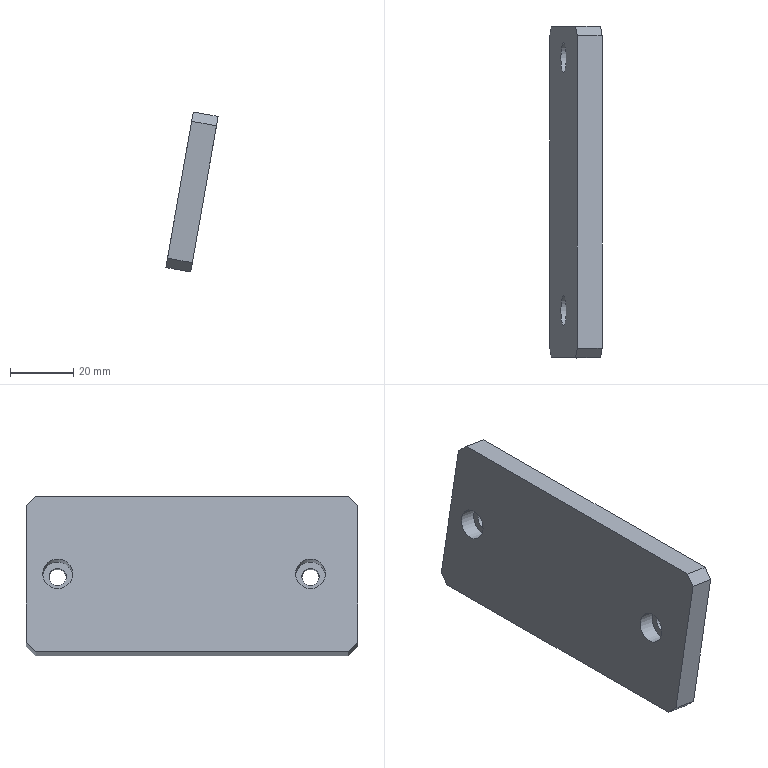Part | STEP file | P011002S003-006 | 1 solid | 16 faces | box 16.561 x 105 x 50.63 mm | volume 40958 mm3 | plane 12 | cylinder 4 | commonest cylinder face diameters 5.5 x2 9.5 x2
STEP:
#1=CARTESIAN_POINT('',(0.,0.,0.));
#2=DIRECTION('',(0.,0.,1.));
#3=DIRECTION('',(1.,0.,0.));
#4=AXIS2_PLACEMENT_3D('',#1,#2,#3);
#5=CARTESIAN_POINT('',(-223.214,6.,16.938));
#6=VERTEX_POINT('',#5);
#7=CARTESIAN_POINT('',(-223.692,6.,14.229));
#8=DIRECTION('',(0.9848,0.,-0.1736));
#9=DIRECTION('',(0.1736,0.,0.9848));
#10=AXIS2_PLACEMENT_3D('',#7,#8,#9);
#11=CIRCLE('',#10,2.75);
#12=CARTESIAN_POINT('',(-220.219,-62.,33.926));
#13=DIRECTION('',(0.9848,0.,-0.1736));
#14=DIRECTION('',(0.,1.,0.));
#15=AXIS2_PLACEMENT_3D('',#12,#13,#14);
#16=PLANE('',#15);
#17=CARTESIAN_POINT('',(68.,-20.));
#18=DIRECTION('',(0.,1.));
#19=AXIS2_PLACEMENT_2D('',#17,#18);
#20=CIRCLE('',#19,2.75);
#21=(GEOMETRIC_REPRESENTATION_CONTEXT(2)PARAMETRIC_REPRESENTATION_CONTEXT()REPRESENTATION_CONTEXT('',''));
#22=DEFINITIONAL_REPRESENTATION('',(#20),#21);
#23=PCURVE('',#16,#22);
#24=CARTESIAN_POINT('',(-231.57,6.,15.619));
#25=DIRECTION('',(0.9848,0.,-0.1736));
#26=DIRECTION('',(0.1736,0.,0.9848));
#27=AXIS2_PLACEMENT_3D('',#24,#25,#26);
#28=CYLINDRICAL_SURFACE('',#27,2.75);
#29=CARTESIAN_POINT('',(0.,8.));
#30=DIRECTION('',(1.,0.));
#31=VECTOR('',#30,1.);
#32=LINE('',#29,#31);
#33=(GEOMETRIC_REPRESENTATION_CONTEXT(2)PARAMETRIC_REPRESENTATION_CONTEXT()REPRESENTATION_CONTEXT('',''));
#34=DEFINITIONAL_REPRESENTATION('',(#32),#33);
#35=PCURVE('',#28,#34);
#36=SURFACE_CURVE('',#11,(#23,#35),.PCURVE_S1.);
#37=EDGE_CURVE('',#6,#6,#36,.T.);
#38=ORIENTED_EDGE('',*,*,#37,.F.);
#39=EDGE_LOOP('',(#38));
#40=FACE_BOUND('',#39,.T.);
#41=CARTESIAN_POINT('',(-219.35,93.,38.85));
#42=VERTEX_POINT('',#41);
#43=CARTESIAN_POINT('',(-219.35,-6.,38.85));
#44=VERTEX_POINT('',#43);
#45=CARTESIAN_POINT('',(-219.35,-62.,38.85));
#46=DIRECTION('',(0.,-1.,0.));
#47=VECTOR('',#46,1.);
#48=LINE('',#45,#47);
#49=CARTESIAN_POINT('',(0.,5.));
#50=DIRECTION('',(-1.,0.));
#51=VECTOR('',#50,1.);
#52=LINE('',#49,#51);
#53=(GEOMETRIC_REPRESENTATION_CONTEXT(2)PARAMETRIC_REPRESENTATION_CONTEXT()REPRESENTATION_CONTEXT('',''));
#54=DEFINITIONAL_REPRESENTATION('',(#52),#53);
#55=PCURVE('',#16,#54);
#56=CARTESIAN_POINT('',(-226.736,-62.,40.152));
#57=DIRECTION('',(0.1736,0.,0.9848));
#58=DIRECTION('',(0.9848,0.,-0.1736));
#59=AXIS2_PLACEMENT_3D('',#56,#57,#58);
#60=PLANE('',#59);
#61=CARTESIAN_POINT('',(7.5,0.));
#62=DIRECTION('',(0.,-1.));
#63=VECTOR('',#62,1.);
#64=LINE('',#61,#63);
#65=(GEOMETRIC_REPRESENTATION_CONTEXT(2)PARAMETRIC_REPRESENTATION_CONTEXT()REPRESENTATION_CONTEXT('',''));
#66=DEFINITIONAL_REPRESENTATION('',(#64),#65);
#67=PCURVE('',#60,#66);
#68=SURFACE_CURVE('',#48,(#55,#67),.PCURVE_S1.);
#69=EDGE_CURVE('',#42,#44,#68,.T.);
#70=ORIENTED_EDGE('',*,*,#69,.T.);
#71=CARTESIAN_POINT('',(-219.871,-9.,35.895));
#72=VERTEX_POINT('',#71);
#73=CARTESIAN_POINT('',(-224.647,-36.5,8.813));
#74=DIRECTION('',(0.1228,0.7071,0.6964));
#75=VECTOR('',#74,1.);
#76=LINE('',#73,#75);
#77=CARTESIAN_POINT('',(25.5,-25.5));
#78=DIRECTION('',(0.7071,0.7071));
#79=VECTOR('',#78,1.);
#80=LINE('',#77,#79);
#81=(GEOMETRIC_REPRESENTATION_CONTEXT(2)PARAMETRIC_REPRESENTATION_CONTEXT()REPRESENTATION_CONTEXT('',''));
#82=DEFINITIONAL_REPRESENTATION('',(#80),#81);
#83=PCURVE('',#16,#82);
#84=CARTESIAN_POINT('',(-200.102,-9.,32.409));
#85=DIRECTION('',(0.1228,-0.7071,0.6964));
#86=DIRECTION('',(0.,-0.7017,-0.7125));
#87=AXIS2_PLACEMENT_3D('',#84,#85,#86);
#88=PLANE('',#87);
#89=CARTESIAN_POINT('',(36.108,-24.732));
#90=DIRECTION('',(-0.9923,0.1237));
#91=VECTOR('',#90,1.);
#92=LINE('',#89,#91);
#93=(GEOMETRIC_REPRESENTATION_CONTEXT(2)PARAMETRIC_REPRESENTATION_CONTEXT()REPRESENTATION_CONTEXT('',''));
#94=DEFINITIONAL_REPRESENTATION('',(#92),#93);
#95=PCURVE('',#88,#94);
#96=SURFACE_CURVE('',#76,(#83,#95),.PCURVE_S1.);
#97=EDGE_CURVE('',#72,#44,#96,.T.);
#98=ORIENTED_EDGE('',*,*,#97,.F.);
#99=CARTESIAN_POINT('',(-227.512,-9.,-7.436));
#100=VERTEX_POINT('',#99);
#101=CARTESIAN_POINT('',(-220.219,-9.,33.926));
#102=DIRECTION('',(-0.1736,0.,-0.9848));
#103=VECTOR('',#102,1.);
#104=LINE('',#101,#103);
#105=CARTESIAN_POINT('',(53.,0.));
#106=DIRECTION('',(0.,-1.));
#107=VECTOR('',#106,1.);
#108=LINE('',#105,#107);
#109=(GEOMETRIC_REPRESENTATION_CONTEXT(2)PARAMETRIC_REPRESENTATION_CONTEXT()REPRESENTATION_CONTEXT('',''));
#110=DEFINITIONAL_REPRESENTATION('',(#108),#109);
#111=PCURVE('',#16,#110);
#112=CARTESIAN_POINT('',(-197.,-9.,50.));
#113=DIRECTION('',(0.,1.,0.));
#114=DIRECTION('',(0.,0.,1.));
#115=AXIS2_PLACEMENT_3D('',#112,#113,#114);
#116=PLANE('',#115);
#117=CARTESIAN_POINT('',(-16.074,-23.219));
#118=DIRECTION('',(-0.9848,-0.1736));
#119=VECTOR('',#118,1.);
#120=LINE('',#117,#119);
#121=(GEOMETRIC_REPRESENTATION_CONTEXT(2)PARAMETRIC_REPRESENTATION_CONTEXT()REPRESENTATION_CONTEXT('',''));
#122=DEFINITIONAL_REPRESENTATION('',(#120),#121);
#123=PCURVE('',#116,#122);
#124=SURFACE_CURVE('',#104,(#111,#123),.PCURVE_S1.);
#125=EDGE_CURVE('',#72,#100,#124,.T.);
#126=ORIENTED_EDGE('',*,*,#125,.T.);
#127=CARTESIAN_POINT('',(-228.033,-6.,-10.391));
#128=VERTEX_POINT('',#127);
#129=CARTESIAN_POINT('',(-219.264,-56.5,39.342));
#130=DIRECTION('',(0.1228,-0.7071,0.6964));
#131=VECTOR('',#130,1.);
#132=LINE('',#129,#131);
#133=CARTESIAN_POINT('',(5.5,5.5));
#134=DIRECTION('',(-0.7071,0.7071));
#135=VECTOR('',#134,1.);
#136=LINE('',#133,#135);
#137=(GEOMETRIC_REPRESENTATION_CONTEXT(2)PARAMETRIC_REPRESENTATION_CONTEXT()REPRESENTATION_CONTEXT('',''));
#138=DEFINITIONAL_REPRESENTATION('',(#136),#137);
#139=PCURVE('',#16,#138);
#140=CARTESIAN_POINT('',(-207.742,-9.,-10.922));
#141=DIRECTION('',(-0.1228,-0.7071,-0.6964));
#142=DIRECTION('',(0.,0.7017,-0.7125));
#143=AXIS2_PLACEMENT_3D('',#140,#141,#142);
#144=PLANE('',#143);
#145=CARTESIAN_POINT('',(-69.143,-11.609));
#146=DIRECTION('',(-0.9923,0.1237));
#147=VECTOR('',#146,1.);
#148=LINE('',#145,#147);
#149=(GEOMETRIC_REPRESENTATION_CONTEXT(2)PARAMETRIC_REPRESENTATION_CONTEXT()REPRESENTATION_CONTEXT('',''));
#150=DEFINITIONAL_REPRESENTATION('',(#148),#149);
#151=PCURVE('',#144,#150);
#152=SURFACE_CURVE('',#132,(#139,#151),.PCURVE_S1.);
#153=EDGE_CURVE('',#128,#100,#152,.T.);
#154=ORIENTED_EDGE('',*,*,#153,.F.);
#155=CARTESIAN_POINT('',(-228.033,93.,-10.391));
#156=VERTEX_POINT('',#155);
#157=CARTESIAN_POINT('',(-228.033,-62.,-10.391));
#158=DIRECTION('',(0.,1.,0.));
#159=VECTOR('',#158,1.);
#160=LINE('',#157,#159);
#161=CARTESIAN_POINT('',(0.,-45.));
#162=DIRECTION('',(1.,0.));
#163=VECTOR('',#162,1.);
#164=LINE('',#161,#163);
#165=(GEOMETRIC_REPRESENTATION_CONTEXT(2)PARAMETRIC_REPRESENTATION_CONTEXT()REPRESENTATION_CONTEXT('',''));
#166=DEFINITIONAL_REPRESENTATION('',(#164),#165);
#167=PCURVE('',#16,#166);
#168=CARTESIAN_POINT('',(-235.419,-62.,-9.088));
#169=DIRECTION('',(-0.1736,0.,-0.9848));
#170=DIRECTION('',(-0.9848,0.,0.1736));
#171=AXIS2_PLACEMENT_3D('',#168,#169,#170);
#172=PLANE('',#171);
#173=CARTESIAN_POINT('',(-7.5,0.));
#174=DIRECTION('',(0.,1.));
#175=VECTOR('',#174,1.);
#176=LINE('',#173,#175);
#177=(GEOMETRIC_REPRESENTATION_CONTEXT(2)PARAMETRIC_REPRESENTATION_CONTEXT()REPRESENTATION_CONTEXT('',''));
#178=DEFINITIONAL_REPRESENTATION('',(#176),#177);
#179=PCURVE('',#172,#178);
#180=SURFACE_CURVE('',#160,(#167,#179),.PCURVE_S1.);
#181=EDGE_CURVE('',#128,#156,#180,.T.);
#182=ORIENTED_EDGE('',*,*,#181,.T.);
#183=CARTESIAN_POINT('',(-227.512,96.,-7.436));
#184=VERTEX_POINT('',#183);
#185=CARTESIAN_POINT('',(-237.583,38.,-64.555));
#186=DIRECTION('',(-0.1228,-0.7071,-0.6964));
#187=VECTOR('',#186,1.);
#188=LINE('',#185,#187);
#189=CARTESIAN_POINT('',(100.,-100.));
#190=DIRECTION('',(-0.7071,-0.7071));
#191=VECTOR('',#190,1.);
#192=LINE('',#189,#191);
#193=(GEOMETRIC_REPRESENTATION_CONTEXT(2)PARAMETRIC_REPRESENTATION_CONTEXT()REPRESENTATION_CONTEXT('',''));
#194=DEFINITIONAL_REPRESENTATION('',(#192),#193);
#195=PCURVE('',#16,#194);
#196=CARTESIAN_POINT('',(-231.451,96.,-6.742));
#197=DIRECTION('',(-0.1228,0.7071,-0.6964));
#198=DIRECTION('',(0.,0.7017,0.7125));
#199=AXIS2_PLACEMENT_3D('',#196,#197,#198);
#200=PLANE('',#199);
#201=CARTESIAN_POINT('',(-81.889,-6.179));
#202=DIRECTION('',(-0.9923,-0.1237));
#203=VECTOR('',#202,1.);
#204=LINE('',#201,#203);
#205=(GEOMETRIC_REPRESENTATION_CONTEXT(2)PARAMETRIC_REPRESENTATION_CONTEXT()REPRESENTATION_CONTEXT('',''));
#206=DEFINITIONAL_REPRESENTATION('',(#204),#205);
#207=PCURVE('',#200,#206);
#208=SURFACE_CURVE('',#188,(#195,#207),.PCURVE_S1.);
#209=EDGE_CURVE('',#184,#156,#208,.T.);
#210=ORIENTED_EDGE('',*,*,#209,.F.);
#211=CARTESIAN_POINT('',(-219.871,96.,35.895));
#212=VERTEX_POINT('',#211);
#213=CARTESIAN_POINT('',(-220.219,96.,33.926));
#214=DIRECTION('',(0.1736,0.,0.9848));
#215=VECTOR('',#214,1.);
#216=LINE('',#213,#215);
#217=CARTESIAN_POINT('',(158.,0.));
#218=DIRECTION('',(0.,1.));
#219=VECTOR('',#218,1.);
#220=LINE('',#217,#219);
#221=(GEOMETRIC_REPRESENTATION_CONTEXT(2)PARAMETRIC_REPRESENTATION_CONTEXT()REPRESENTATION_CONTEXT('',''));
#222=DEFINITIONAL_REPRESENTATION('',(#220),#221);
#223=PCURVE('',#16,#222);
#224=CARTESIAN_POINT('',(-227.631,96.,14.924));
#225=DIRECTION('',(0.,-1.,0.));
#226=DIRECTION('',(0.,0.,-1.));
#227=AXIS2_PLACEMENT_3D('',#224,#225,#226);
#228=PLANE('',#227);
#229=CARTESIAN_POINT('',(-19.002,7.412));
#230=DIRECTION('',(-0.9848,0.1736));
#231=VECTOR('',#230,1.);
#232=LINE('',#229,#231);
#233=(GEOMETRIC_REPRESENTATION_CONTEXT(2)PARAMETRIC_REPRESENTATION_CONTEXT()REPRESENTATION_CONTEXT('',''));
#234=DEFINITIONAL_REPRESENTATION('',(#232),#233);
#235=PCURVE('',#228,#234);
#236=SURFACE_CURVE('',#216,(#223,#235),.PCURVE_S1.);
#237=EDGE_CURVE('',#184,#212,#236,.T.);
#238=ORIENTED_EDGE('',*,*,#237,.T.);
#239=CARTESIAN_POINT('',(-206.327,18.,112.71));
#240=DIRECTION('',(-0.1228,0.7071,-0.6964));
#241=VECTOR('',#240,1.);
#242=LINE('',#239,#241);
#243=CARTESIAN_POINT('',(80.,80.));
#244=DIRECTION('',(0.7071,-0.7071));
#245=VECTOR('',#244,1.);
#246=LINE('',#243,#245);
#247=(GEOMETRIC_REPRESENTATION_CONTEXT(2)PARAMETRIC_REPRESENTATION_CONTEXT()REPRESENTATION_CONTEXT('',''));
#248=DEFINITIONAL_REPRESENTATION('',(#246),#247);
#249=PCURVE('',#16,#248);
#250=CARTESIAN_POINT('',(-223.811,96.,36.59));
#251=DIRECTION('',(0.1228,0.7071,0.6964));
#252=DIRECTION('',(0.,-0.7017,0.7125));
#253=AXIS2_PLACEMENT_3D('',#250,#251,#252);
#254=PLANE('',#253);
#255=CARTESIAN_POINT('',(108.966,17.617));
#256=DIRECTION('',(-0.9923,-0.1237));
#257=VECTOR('',#256,1.);
#258=LINE('',#255,#257);
#259=(GEOMETRIC_REPRESENTATION_CONTEXT(2)PARAMETRIC_REPRESENTATION_CONTEXT()REPRESENTATION_CONTEXT('',''));
#260=DEFINITIONAL_REPRESENTATION('',(#258),#259);
#261=PCURVE('',#254,#260);
#262=SURFACE_CURVE('',#242,(#249,#261),.PCURVE_S1.);
#263=EDGE_CURVE('',#42,#212,#262,.T.);
#264=ORIENTED_EDGE('',*,*,#263,.F.);
#265=EDGE_LOOP('',(#70,#98,#126,#154,#182,#210,#238,#264));
#266=FACE_BOUND('',#265,.T.);
#267=CARTESIAN_POINT('',(-223.214,86.,16.938));
#268=VERTEX_POINT('',#267);
#269=CARTESIAN_POINT('',(-223.692,86.,14.229));
#270=DIRECTION('',(0.9848,0.,-0.1736));
#271=DIRECTION('',(0.1736,0.,0.9848));
#272=AXIS2_PLACEMENT_3D('',#269,#270,#271);
#273=CIRCLE('',#272,2.75);
#274=CARTESIAN_POINT('',(148.,-20.));
#275=DIRECTION('',(0.,1.));
#276=AXIS2_PLACEMENT_2D('',#274,#275);
#277=CIRCLE('',#276,2.75);
#278=(GEOMETRIC_REPRESENTATION_CONTEXT(2)PARAMETRIC_REPRESENTATION_CONTEXT()REPRESENTATION_CONTEXT('',''));
#279=DEFINITIONAL_REPRESENTATION('',(#277),#278);
#280=PCURVE('',#16,#279);
#281=CARTESIAN_POINT('',(-231.57,86.,15.619));
#282=DIRECTION('',(0.9848,0.,-0.1736));
#283=DIRECTION('',(0.1736,0.,0.9848));
#284=AXIS2_PLACEMENT_3D('',#281,#282,#283);
#285=CYLINDRICAL_SURFACE('',#284,2.75);
#286=CARTESIAN_POINT('',(0.,8.));
#287=DIRECTION('',(1.,0.));
#288=VECTOR('',#287,1.);
#289=LINE('',#286,#288);
#290=(GEOMETRIC_REPRESENTATION_CONTEXT(2)PARAMETRIC_REPRESENTATION_CONTEXT()REPRESENTATION_CONTEXT('',''));
#291=DEFINITIONAL_REPRESENTATION('',(#289),#290);
#292=PCURVE('',#285,#291);
#293=SURFACE_CURVE('',#273,(#280,#292),.PCURVE_S1.);
#294=EDGE_CURVE('',#268,#268,#293,.T.);
#295=ORIENTED_EDGE('',*,*,#294,.F.);
#296=EDGE_LOOP('',(#295));
#297=FACE_BOUND('',#296,.T.);
#298=ADVANCED_FACE('',(#40,#266,#297),#16,.T.);
#299=CARTESIAN_POINT('',(-230.745,86.,20.296));
#300=VERTEX_POINT('',#299);
#301=CARTESIAN_POINT('',(-231.57,86.,15.619));
#302=DIRECTION('',(0.9848,0.,-0.1736));
#303=DIRECTION('',(0.1736,0.,0.9848));
#304=AXIS2_PLACEMENT_3D('',#301,#302,#303);
#305=CIRCLE('',#304,4.75);
#306=CARTESIAN_POINT('',(-228.097,-62.,35.315));
#307=DIRECTION('',(-0.9848,0.,0.1736));
#308=DIRECTION('',(0.,-1.,0.));
#309=AXIS2_PLACEMENT_3D('',#306,#307,#308);
#310=PLANE('',#309);
#311=CARTESIAN_POINT('',(-148.,-15.25));
#312=CARTESIAN_POINT('',(-139.773,-15.25));
#313=CARTESIAN_POINT('',(-143.886,-22.375));
#314=CARTESIAN_POINT('',(-148.,-29.5));
#315=CARTESIAN_POINT('',(-152.114,-22.375));
#316=CARTESIAN_POINT('',(-156.227,-15.25));
#317=CARTESIAN_POINT('',(-148.,-15.25));
#318=(BOUNDED_CURVE()B_SPLINE_CURVE(2,(#311,#312,#313,#314,#315,#316,#317),.UNSPECIFIED.,.T.,.F.)B_SPLINE_CURVE_WITH_KNOTS((1,2,2,2,2,1),(-2.094,0.,2.094,4.189,6.283,8.378),.UNSPECIFIED.)CURVE()GEOMETRIC_REPRESENTATION_ITEM()RATIONAL_B_SPLINE_CURVE((1.,0.5,1.,0.5,1.,0.5,1.))REPRESENTATION_ITEM(''));
#319=(GEOMETRIC_REPRESENTATION_CONTEXT(2)PARAMETRIC_REPRESENTATION_CONTEXT()REPRESENTATION_CONTEXT('',''));
#320=DEFINITIONAL_REPRESENTATION('',(#318),#319);
#321=PCURVE('',#310,#320);
#322=CARTESIAN_POINT('',(-231.57,86.,15.619));
#323=DIRECTION('',(0.9848,0.,-0.1736));
#324=DIRECTION('',(0.1736,0.,0.9848));
#325=AXIS2_PLACEMENT_3D('',#322,#323,#324);
#326=CYLINDRICAL_SURFACE('',#325,4.75);
#327=CARTESIAN_POINT('',(0.,0.));
#328=DIRECTION('',(1.,0.));
#329=VECTOR('',#328,1.);
#330=LINE('',#327,#329);
#331=(GEOMETRIC_REPRESENTATION_CONTEXT(2)PARAMETRIC_REPRESENTATION_CONTEXT()REPRESENTATION_CONTEXT('',''));
#332=DEFINITIONAL_REPRESENTATION('',(#330),#331);
#333=PCURVE('',#326,#332);
#334=SURFACE_CURVE('',#305,(#321,#333),.PCURVE_S1.);
#335=EDGE_CURVE('',#300,#300,#334,.T.);
#336=ORIENTED_EDGE('',*,*,#335,.T.);
#337=EDGE_LOOP('',(#336));
#338=FACE_BOUND('',#337,.T.);
#339=CARTESIAN_POINT('',(-230.745,6.,20.296));
#340=VERTEX_POINT('',#339);
#341=CARTESIAN_POINT('',(-231.57,6.,15.619));
#342=DIRECTION('',(0.9848,0.,-0.1736));
#343=DIRECTION('',(0.1736,0.,0.9848));
#344=AXIS2_PLACEMENT_3D('',#341,#342,#343);
#345=CIRCLE('',#344,4.75);
#346=CARTESIAN_POINT('',(-68.,-15.25));
#347=CARTESIAN_POINT('',(-59.773,-15.25));
#348=CARTESIAN_POINT('',(-63.886,-22.375));
#349=CARTESIAN_POINT('',(-68.,-29.5));
#350=CARTESIAN_POINT('',(-72.114,-22.375));
#351=CARTESIAN_POINT('',(-76.227,-15.25));
#352=CARTESIAN_POINT('',(-68.,-15.25));
#353=(BOUNDED_CURVE()B_SPLINE_CURVE(2,(#346,#347,#348,#349,#350,#351,#352),.UNSPECIFIED.,.T.,.F.)B_SPLINE_CURVE_WITH_KNOTS((1,2,2,2,2,1),(-2.094,0.,2.094,4.189,6.283,8.378),.UNSPECIFIED.)CURVE()GEOMETRIC_REPRESENTATION_ITEM()RATIONAL_B_SPLINE_CURVE((1.,0.5,1.,0.5,1.,0.5,1.))REPRESENTATION_ITEM(''));
#354=(GEOMETRIC_REPRESENTATION_CONTEXT(2)PARAMETRIC_REPRESENTATION_CONTEXT()REPRESENTATION_CONTEXT('',''));
#355=DEFINITIONAL_REPRESENTATION('',(#353),#354);
#356=PCURVE('',#310,#355);
#357=CARTESIAN_POINT('',(-231.57,6.,15.619));
#358=DIRECTION('',(0.9848,0.,-0.1736));
#359=DIRECTION('',(0.1736,0.,0.9848));
#360=AXIS2_PLACEMENT_3D('',#357,#358,#359);
#361=CYLINDRICAL_SURFACE('',#360,4.75);
#362=CARTESIAN_POINT('',(0.,0.));
#363=DIRECTION('',(1.,0.));
#364=VECTOR('',#363,1.);
#365=LINE('',#362,#364);
#366=(GEOMETRIC_REPRESENTATION_CONTEXT(2)PARAMETRIC_REPRESENTATION_CONTEXT()REPRESENTATION_CONTEXT('',''));
#367=DEFINITIONAL_REPRESENTATION('',(#365),#366);
#368=PCURVE('',#361,#367);
#369=SURFACE_CURVE('',#345,(#356,#368),.PCURVE_S1.);
#370=EDGE_CURVE('',#340,#340,#369,.T.);
#371=ORIENTED_EDGE('',*,*,#370,.T.);
#372=EDGE_LOOP('',(#371));
#373=FACE_BOUND('',#372,.T.);
#374=CARTESIAN_POINT('',(-227.75,96.,37.284));
#375=VERTEX_POINT('',#374);
#376=CARTESIAN_POINT('',(-235.39,96.,-6.047));
#377=VERTEX_POINT('',#376);
#378=CARTESIAN_POINT('',(-228.097,96.,35.315));
#379=DIRECTION('',(-0.1736,0.,-0.9848));
#380=VECTOR('',#379,1.);
#381=LINE('',#378,#380);
#382=CARTESIAN_POINT('',(-158.,0.));
#383=DIRECTION('',(0.,-1.));
#384=VECTOR('',#383,1.);
#385=LINE('',#382,#384);
#386=(GEOMETRIC_REPRESENTATION_CONTEXT(2)PARAMETRIC_REPRESENTATION_CONTEXT()REPRESENTATION_CONTEXT('',''));
#387=DEFINITIONAL_REPRESENTATION('',(#385),#386);
#388=PCURVE('',#310,#387);
#389=CARTESIAN_POINT('',(-20.391,-0.4663));
#390=DIRECTION('',(0.9848,-0.1736));
#391=VECTOR('',#390,1.);
#392=LINE('',#389,#391);
#393=(GEOMETRIC_REPRESENTATION_CONTEXT(2)PARAMETRIC_REPRESENTATION_CONTEXT()REPRESENTATION_CONTEXT('',''));
#394=DEFINITIONAL_REPRESENTATION('',(#392),#393);
#395=PCURVE('',#228,#394);
#396=SURFACE_CURVE('',#381,(#388,#395),.PCURVE_S1.);
#397=EDGE_CURVE('',#375,#377,#396,.T.);
#398=ORIENTED_EDGE('',*,*,#397,.T.);
#399=CARTESIAN_POINT('',(-235.911,93.,-9.002));
#400=VERTEX_POINT('',#399);
#401=CARTESIAN_POINT('',(-245.462,38.,-63.166));
#402=DIRECTION('',(0.1228,0.7071,0.6964));
#403=VECTOR('',#402,1.);
#404=LINE('',#401,#403);
#405=CARTESIAN_POINT('',(-100.,-100.));
#406=DIRECTION('',(-0.7071,0.7071));
#407=VECTOR('',#406,1.);
#408=LINE('',#405,#407);
#409=(GEOMETRIC_REPRESENTATION_CONTEXT(2)PARAMETRIC_REPRESENTATION_CONTEXT()REPRESENTATION_CONTEXT('',''));
#410=DEFINITIONAL_REPRESENTATION('',(#408),#409);
#411=PCURVE('',#310,#410);
#412=CARTESIAN_POINT('',(-80.899,-14.118));
#413=DIRECTION('',(0.9923,0.1237));
#414=VECTOR('',#413,1.);
#415=LINE('',#412,#414);
#416=(GEOMETRIC_REPRESENTATION_CONTEXT(2)PARAMETRIC_REPRESENTATION_CONTEXT()REPRESENTATION_CONTEXT('',''));
#417=DEFINITIONAL_REPRESENTATION('',(#415),#416);
#418=PCURVE('',#200,#417);
#419=SURFACE_CURVE('',#404,(#411,#418),.PCURVE_S1.);
#420=EDGE_CURVE('',#400,#377,#419,.T.);
#421=ORIENTED_EDGE('',*,*,#420,.F.);
#422=CARTESIAN_POINT('',(-235.911,-6.,-9.002));
#423=VERTEX_POINT('',#422);
#424=CARTESIAN_POINT('',(-235.911,-62.,-9.002));
#425=DIRECTION('',(0.,-1.,0.));
#426=VECTOR('',#425,1.);
#427=LINE('',#424,#426);
#428=CARTESIAN_POINT('',(0.,-45.));
#429=DIRECTION('',(1.,0.));
#430=VECTOR('',#429,1.);
#431=LINE('',#428,#430);
#432=(GEOMETRIC_REPRESENTATION_CONTEXT(2)PARAMETRIC_REPRESENTATION_CONTEXT()REPRESENTATION_CONTEXT('',''));
#433=DEFINITIONAL_REPRESENTATION('',(#431),#432);
#434=PCURVE('',#310,#433);
#435=CARTESIAN_POINT('',(0.5,0.));
#436=DIRECTION('',(0.,-1.));
#437=VECTOR('',#436,1.);
#438=LINE('',#435,#437);
#439=(GEOMETRIC_REPRESENTATION_CONTEXT(2)PARAMETRIC_REPRESENTATION_CONTEXT()REPRESENTATION_CONTEXT('',''));
#440=DEFINITIONAL_REPRESENTATION('',(#438),#439);
#441=PCURVE('',#172,#440);
#442=SURFACE_CURVE('',#427,(#434,#441),.PCURVE_S1.);
#443=EDGE_CURVE('',#400,#423,#442,.T.);
#444=ORIENTED_EDGE('',*,*,#443,.T.);
#445=CARTESIAN_POINT('',(-235.39,-9.,-6.047));
#446=VERTEX_POINT('',#445);
#447=CARTESIAN_POINT('',(-227.142,-56.5,40.731));
#448=DIRECTION('',(-0.1228,0.7071,-0.6964));
#449=VECTOR('',#448,1.);
#450=LINE('',#447,#449);
#451=CARTESIAN_POINT('',(-5.5,5.5));
#452=DIRECTION('',(-0.7071,-0.7071));
#453=VECTOR('',#452,1.);
#454=LINE('',#451,#453);
#455=(GEOMETRIC_REPRESENTATION_CONTEXT(2)PARAMETRIC_REPRESENTATION_CONTEXT()REPRESENTATION_CONTEXT('',''));
#456=DEFINITIONAL_REPRESENTATION('',(#454),#455);
#457=PCURVE('',#310,#456);
#458=CARTESIAN_POINT('',(-70.133,-19.548));
#459=DIRECTION('',(0.9923,-0.1237));
#460=VECTOR('',#459,1.);
#461=LINE('',#458,#460);
#462=(GEOMETRIC_REPRESENTATION_CONTEXT(2)PARAMETRIC_REPRESENTATION_CONTEXT()REPRESENTATION_CONTEXT('',''));
#463=DEFINITIONAL_REPRESENTATION('',(#461),#462);
#464=PCURVE('',#144,#463);
#465=SURFACE_CURVE('',#450,(#457,#464),.PCURVE_S1.);
#466=EDGE_CURVE('',#446,#423,#465,.T.);
#467=ORIENTED_EDGE('',*,*,#466,.F.);
#468=CARTESIAN_POINT('',(-227.75,-9.,37.284));
#469=VERTEX_POINT('',#468);
#470=CARTESIAN_POINT('',(-228.097,-9.,35.315));
#471=DIRECTION('',(0.1736,0.,0.9848));
#472=VECTOR('',#471,1.);
#473=LINE('',#470,#472);
#474=CARTESIAN_POINT('',(-53.,0.));
#475=DIRECTION('',(0.,1.));
#476=VECTOR('',#475,1.);
#477=LINE('',#474,#476);
#478=(GEOMETRIC_REPRESENTATION_CONTEXT(2)PARAMETRIC_REPRESENTATION_CONTEXT()REPRESENTATION_CONTEXT('',''));
#479=DEFINITIONAL_REPRESENTATION('',(#477),#478);
#480=PCURVE('',#310,#479);
#481=CARTESIAN_POINT('',(-14.685,-31.097));
#482=DIRECTION('',(0.9848,0.1736));
#483=VECTOR('',#482,1.);
#484=LINE('',#481,#483);
#485=(GEOMETRIC_REPRESENTATION_CONTEXT(2)PARAMETRIC_REPRESENTATION_CONTEXT()REPRESENTATION_CONTEXT('',''));
#486=DEFINITIONAL_REPRESENTATION('',(#484),#485);
#487=PCURVE('',#116,#486);
#488=SURFACE_CURVE('',#473,(#480,#487),.PCURVE_S1.);
#489=EDGE_CURVE('',#446,#469,#488,.T.);
#490=ORIENTED_EDGE('',*,*,#489,.T.);
#491=CARTESIAN_POINT('',(-227.229,-6.,40.239));
#492=VERTEX_POINT('',#491);
#493=CARTESIAN_POINT('',(-232.525,-36.5,10.202));
#494=DIRECTION('',(-0.1228,-0.7071,-0.6964));
#495=VECTOR('',#494,1.);
#496=LINE('',#493,#495);
#497=CARTESIAN_POINT('',(-25.5,-25.5));
#498=DIRECTION('',(0.7071,-0.7071));
#499=VECTOR('',#498,1.);
#500=LINE('',#497,#499);
#501=(GEOMETRIC_REPRESENTATION_CONTEXT(2)PARAMETRIC_REPRESENTATION_CONTEXT()REPRESENTATION_CONTEXT('',''));
#502=DEFINITIONAL_REPRESENTATION('',(#500),#501);
#503=PCURVE('',#310,#502);
#504=CARTESIAN_POINT('',(35.119,-32.671));
#505=DIRECTION('',(0.9923,-0.1237));
#506=VECTOR('',#505,1.);
#507=LINE('',#504,#506);
#508=(GEOMETRIC_REPRESENTATION_CONTEXT(2)PARAMETRIC_REPRESENTATION_CONTEXT()REPRESENTATION_CONTEXT('',''));
#509=DEFINITIONAL_REPRESENTATION('',(#507),#508);
#510=PCURVE('',#88,#509);
#511=SURFACE_CURVE('',#496,(#503,#510),.PCURVE_S1.);
#512=EDGE_CURVE('',#492,#469,#511,.T.);
#513=ORIENTED_EDGE('',*,*,#512,.F.);
#514=CARTESIAN_POINT('',(-227.229,93.,40.239));
#515=VERTEX_POINT('',#514);
#516=CARTESIAN_POINT('',(-227.229,-62.,40.239));
#517=DIRECTION('',(0.,1.,0.));
#518=VECTOR('',#517,1.);
#519=LINE('',#516,#518);
#520=CARTESIAN_POINT('',(0.,5.));
#521=DIRECTION('',(-1.,0.));
#522=VECTOR('',#521,1.);
#523=LINE('',#520,#522);
#524=(GEOMETRIC_REPRESENTATION_CONTEXT(2)PARAMETRIC_REPRESENTATION_CONTEXT()REPRESENTATION_CONTEXT('',''));
#525=DEFINITIONAL_REPRESENTATION('',(#523),#524);
#526=PCURVE('',#310,#525);
#527=CARTESIAN_POINT('',(-0.5,0.));
#528=DIRECTION('',(0.,1.));
#529=VECTOR('',#528,1.);
#530=LINE('',#527,#529);
#531=(GEOMETRIC_REPRESENTATION_CONTEXT(2)PARAMETRIC_REPRESENTATION_CONTEXT()REPRESENTATION_CONTEXT('',''));
#532=DEFINITIONAL_REPRESENTATION('',(#530),#531);
#533=PCURVE('',#60,#532);
#534=SURFACE_CURVE('',#519,(#526,#533),.PCURVE_S1.);
#535=EDGE_CURVE('',#492,#515,#534,.T.);
#536=ORIENTED_EDGE('',*,*,#535,.T.);
#537=CARTESIAN_POINT('',(-214.205,18.,114.099));
#538=DIRECTION('',(0.1228,-0.7071,0.6964));
#539=VECTOR('',#538,1.);
#540=LINE('',#537,#539);
#541=CARTESIAN_POINT('',(-80.,80.));
#542=DIRECTION('',(0.7071,0.7071));
#543=VECTOR('',#542,1.);
#544=LINE('',#541,#543);
#545=(GEOMETRIC_REPRESENTATION_CONTEXT(2)PARAMETRIC_REPRESENTATION_CONTEXT()REPRESENTATION_CONTEXT('',''));
#546=DEFINITIONAL_REPRESENTATION('',(#544),#545);
#547=PCURVE('',#310,#546);
#548=CARTESIAN_POINT('',(109.956,9.679));
#549=DIRECTION('',(0.9923,0.1237));
#550=VECTOR('',#549,1.);
#551=LINE('',#548,#550);
#552=(GEOMETRIC_REPRESENTATION_CONTEXT(2)PARAMETRIC_REPRESENTATION_CONTEXT()REPRESENTATION_CONTEXT('',''));
#553=DEFINITIONAL_REPRESENTATION('',(#551),#552);
#554=PCURVE('',#254,#553);
#555=SURFACE_CURVE('',#540,(#547,#554),.PCURVE_S1.);
#556=EDGE_CURVE('',#375,#515,#555,.T.);
#557=ORIENTED_EDGE('',*,*,#556,.F.);
#558=EDGE_LOOP('',(#398,#421,#444,#467,#490,#513,#536,#557));
#559=FACE_BOUND('',#558,.T.);
#560=ADVANCED_FACE('',(#338,#373,#559),#310,.T.);
#561=ORIENTED_EDGE('',*,*,#535,.F.);
#562=CARTESIAN_POINT('',(-227.229,-6.,40.239));
#563=DIRECTION('',(-0.9848,0.,0.1736));
#564=VECTOR('',#563,1.);
#565=LINE('',#562,#564);
#566=CARTESIAN_POINT('',(-0.5,56.));
#567=DIRECTION('',(-1.,0.));
#568=VECTOR('',#567,1.);
#569=LINE('',#566,#568);
#570=(GEOMETRIC_REPRESENTATION_CONTEXT(2)PARAMETRIC_REPRESENTATION_CONTEXT()REPRESENTATION_CONTEXT('',''));
#571=DEFINITIONAL_REPRESENTATION('',(#569),#570);
#572=PCURVE('',#60,#571);
#573=CARTESIAN_POINT('',(-7.684,-27.334));
#574=DIRECTION('',(-0.1237,-0.9923));
#575=VECTOR('',#574,1.);
#576=LINE('',#573,#575);
#577=(GEOMETRIC_REPRESENTATION_CONTEXT(2)PARAMETRIC_REPRESENTATION_CONTEXT()REPRESENTATION_CONTEXT('',''));
#578=DEFINITIONAL_REPRESENTATION('',(#576),#577);
#579=PCURVE('',#88,#578);
#580=SURFACE_CURVE('',#565,(#572,#579),.PCURVE_S1.);
#581=EDGE_CURVE('',#44,#492,#580,.T.);
#582=ORIENTED_EDGE('',*,*,#581,.F.);
#583=ORIENTED_EDGE('',*,*,#69,.F.);
#584=CARTESIAN_POINT('',(-219.35,93.,38.85));
#585=DIRECTION('',(0.9848,0.,-0.1736));
#586=VECTOR('',#585,1.);
#587=LINE('',#584,#586);
#588=CARTESIAN_POINT('',(7.5,155.));
#589=DIRECTION('',(1.,0.));
#590=VECTOR('',#589,1.);
#591=LINE('',#588,#590);
#592=(GEOMETRIC_REPRESENTATION_CONTEXT(2)PARAMETRIC_REPRESENTATION_CONTEXT()REPRESENTATION_CONTEXT('',''));
#593=DEFINITIONAL_REPRESENTATION('',(#591),#592);
#594=PCURVE('',#60,#593);
#595=CARTESIAN_POINT('',(3.715,4.494));
#596=DIRECTION('',(-0.1237,0.9923));
#597=VECTOR('',#596,1.);
#598=LINE('',#595,#597);
#599=(GEOMETRIC_REPRESENTATION_CONTEXT(2)PARAMETRIC_REPRESENTATION_CONTEXT()REPRESENTATION_CONTEXT('',''));
#600=DEFINITIONAL_REPRESENTATION('',(#598),#599);
#601=PCURVE('',#254,#600);
#602=SURFACE_CURVE('',#587,(#594,#601),.PCURVE_S1.);
#603=EDGE_CURVE('',#515,#42,#602,.T.);
#604=ORIENTED_EDGE('',*,*,#603,.F.);
#605=EDGE_LOOP('',(#561,#582,#583,#604));
#606=FACE_BOUND('',#605,.T.);
#607=ADVANCED_FACE('',(#606),#60,.T.);
#608=ORIENTED_EDGE('',*,*,#181,.F.);
#609=CARTESIAN_POINT('',(-228.033,-6.,-10.391));
#610=DIRECTION('',(0.9848,0.,-0.1736));
#611=VECTOR('',#610,1.);
#612=LINE('',#609,#611);
#613=CARTESIAN_POINT('',(-7.5,56.));
#614=DIRECTION('',(-1.,0.));
#615=VECTOR('',#614,1.);
#616=LINE('',#613,#615);
#617=(GEOMETRIC_REPRESENTATION_CONTEXT(2)PARAMETRIC_REPRESENTATION_CONTEXT()REPRESENTATION_CONTEXT('',''));
#618=DEFINITIONAL_REPRESENTATION('',(#616),#617);
#619=PCURVE('',#172,#618);
#620=CARTESIAN_POINT('',(1.726,-20.445));
#621=DIRECTION('',(0.1237,0.9923));
#622=VECTOR('',#621,1.);
#623=LINE('',#620,#622);
#624=(GEOMETRIC_REPRESENTATION_CONTEXT(2)PARAMETRIC_REPRESENTATION_CONTEXT()REPRESENTATION_CONTEXT('',''));
#625=DEFINITIONAL_REPRESENTATION('',(#623),#624);
#626=PCURVE('',#144,#625);
#627=SURFACE_CURVE('',#612,(#619,#626),.PCURVE_S1.);
#628=EDGE_CURVE('',#423,#128,#627,.T.);
#629=ORIENTED_EDGE('',*,*,#628,.F.);
#630=ORIENTED_EDGE('',*,*,#443,.F.);
#631=CARTESIAN_POINT('',(-235.911,93.,-9.002));
#632=DIRECTION('',(-0.9848,0.,0.1736));
#633=VECTOR('',#632,1.);
#634=LINE('',#631,#633);
#635=CARTESIAN_POINT('',(0.5,155.));
#636=DIRECTION('',(1.,0.));
#637=VECTOR('',#636,1.);
#638=LINE('',#635,#637);
#639=(GEOMETRIC_REPRESENTATION_CONTEXT(2)PARAMETRIC_REPRESENTATION_CONTEXT()REPRESENTATION_CONTEXT('',''));
#640=DEFINITIONAL_REPRESENTATION('',(#638),#639);
#641=PCURVE('',#172,#640);
#642=CARTESIAN_POINT('',(-3.715,-4.494));
#643=DIRECTION('',(0.1237,-0.9923));
#644=VECTOR('',#643,1.);
#645=LINE('',#642,#644);
#646=(GEOMETRIC_REPRESENTATION_CONTEXT(2)PARAMETRIC_REPRESENTATION_CONTEXT()REPRESENTATION_CONTEXT('',''));
#647=DEFINITIONAL_REPRESENTATION('',(#645),#646);
#648=PCURVE('',#200,#647);
#649=SURFACE_CURVE('',#634,(#641,#648),.PCURVE_S1.);
#650=EDGE_CURVE('',#156,#400,#649,.T.);
#651=ORIENTED_EDGE('',*,*,#650,.F.);
#652=EDGE_LOOP('',(#608,#629,#630,#651));
#653=FACE_BOUND('',#652,.T.);
#654=ADVANCED_FACE('',(#653),#172,.T.);
#655=ORIENTED_EDGE('',*,*,#125,.F.);
#656=CARTESIAN_POINT('',(-219.871,-9.,35.895));
#657=DIRECTION('',(0.9848,0.,-0.1736));
#658=VECTOR('',#657,1.);
#659=LINE('',#656,#658);
#660=CARTESIAN_POINT('',(-14.105,-22.871));
#661=DIRECTION('',(-0.1736,0.9848));
#662=VECTOR('',#661,1.);
#663=LINE('',#660,#662);
#664=(GEOMETRIC_REPRESENTATION_CONTEXT(2)PARAMETRIC_REPRESENTATION_CONTEXT()REPRESENTATION_CONTEXT('',''));
#665=DEFINITIONAL_REPRESENTATION('',(#663),#664);
#666=PCURVE('',#116,#665);
#667=CARTESIAN_POINT('',(-2.484,-19.92));
#668=DIRECTION('',(0.1237,0.9923));
#669=VECTOR('',#668,1.);
#670=LINE('',#667,#669);
#671=(GEOMETRIC_REPRESENTATION_CONTEXT(2)PARAMETRIC_REPRESENTATION_CONTEXT()REPRESENTATION_CONTEXT('',''));
#672=DEFINITIONAL_REPRESENTATION('',(#670),#671);
#673=PCURVE('',#88,#672);
#674=SURFACE_CURVE('',#659,(#666,#673),.PCURVE_S1.);
#675=EDGE_CURVE('',#469,#72,#674,.T.);
#676=ORIENTED_EDGE('',*,*,#675,.F.);
#677=ORIENTED_EDGE('',*,*,#489,.F.);
#678=CARTESIAN_POINT('',(-235.39,-9.,-6.047));
#679=DIRECTION('',(-0.9848,0.,0.1736));
#680=VECTOR('',#679,1.);
#681=LINE('',#678,#680);
#682=CARTESIAN_POINT('',(-56.047,-38.39));
#683=DIRECTION('',(0.1736,-0.9848));
#684=VECTOR('',#683,1.);
#685=LINE('',#682,#684);
#686=(GEOMETRIC_REPRESENTATION_CONTEXT(2)PARAMETRIC_REPRESENTATION_CONTEXT()REPRESENTATION_CONTEXT('',''));
#687=DEFINITIONAL_REPRESENTATION('',(#685),#686);
#688=PCURVE('',#116,#687);
#689=CARTESIAN_POINT('',(-3.474,-27.859));
#690=DIRECTION('',(-0.1237,-0.9923));
#691=VECTOR('',#690,1.);
#692=LINE('',#689,#691);
#693=(GEOMETRIC_REPRESENTATION_CONTEXT(2)PARAMETRIC_REPRESENTATION_CONTEXT()REPRESENTATION_CONTEXT('',''));
#694=DEFINITIONAL_REPRESENTATION('',(#692),#693);
#695=PCURVE('',#144,#694);
#696=SURFACE_CURVE('',#681,(#688,#695),.PCURVE_S1.);
#697=EDGE_CURVE('',#100,#446,#696,.T.);
#698=ORIENTED_EDGE('',*,*,#697,.F.);
#699=EDGE_LOOP('',(#655,#676,#677,#698));
#700=FACE_BOUND('',#699,.T.);
#701=ADVANCED_FACE('',(#700),#116,.F.);
#702=ORIENTED_EDGE('',*,*,#237,.F.);
#703=CARTESIAN_POINT('',(-227.512,96.,-7.436));
#704=DIRECTION('',(0.9848,0.,-0.1736));
#705=VECTOR('',#704,1.);
#706=LINE('',#703,#705);
#707=CARTESIAN_POINT('',(22.36,0.119));
#708=DIRECTION('',(0.1736,0.9848));
#709=VECTOR('',#708,1.);
#710=LINE('',#707,#709);
#711=(GEOMETRIC_REPRESENTATION_CONTEXT(2)PARAMETRIC_REPRESENTATION_CONTEXT()REPRESENTATION_CONTEXT('',''));
#712=DEFINITIONAL_REPRESENTATION('',(#710),#711);
#713=PCURVE('',#228,#712);
#714=CARTESIAN_POINT('',(-0.4949,3.969));
#715=DIRECTION('',(-0.1237,0.9923));
#716=VECTOR('',#715,1.);
#717=LINE('',#714,#716);
#718=(GEOMETRIC_REPRESENTATION_CONTEXT(2)PARAMETRIC_REPRESENTATION_CONTEXT()REPRESENTATION_CONTEXT('',''));
#719=DEFINITIONAL_REPRESENTATION('',(#717),#718);
#720=PCURVE('',#200,#719);
#721=SURFACE_CURVE('',#706,(#713,#720),.PCURVE_S1.);
#722=EDGE_CURVE('',#377,#184,#721,.T.);
#723=ORIENTED_EDGE('',*,*,#722,.F.);
#724=ORIENTED_EDGE('',*,*,#397,.F.);
#725=CARTESIAN_POINT('',(-227.75,96.,37.284));
#726=DIRECTION('',(-0.9848,0.,0.1736));
#727=VECTOR('',#726,1.);
#728=LINE('',#725,#727);
#729=CARTESIAN_POINT('',(-22.36,-0.119));
#730=DIRECTION('',(-0.1736,-0.9848));
#731=VECTOR('',#730,1.);
#732=LINE('',#729,#731);
#733=(GEOMETRIC_REPRESENTATION_CONTEXT(2)PARAMETRIC_REPRESENTATION_CONTEXT()REPRESENTATION_CONTEXT('',''));
#734=DEFINITIONAL_REPRESENTATION('',(#732),#733);
#735=PCURVE('',#228,#734);
#736=CARTESIAN_POINT('',(0.4949,-3.969));
#737=DIRECTION('',(0.1237,-0.9923));
#738=VECTOR('',#737,1.);
#739=LINE('',#736,#738);
#740=(GEOMETRIC_REPRESENTATION_CONTEXT(2)PARAMETRIC_REPRESENTATION_CONTEXT()REPRESENTATION_CONTEXT('',''));
#741=DEFINITIONAL_REPRESENTATION('',(#739),#740);
#742=PCURVE('',#254,#741);
#743=SURFACE_CURVE('',#728,(#735,#742),.PCURVE_S1.);
#744=EDGE_CURVE('',#212,#375,#743,.T.);
#745=ORIENTED_EDGE('',*,*,#744,.F.);
#746=EDGE_LOOP('',(#702,#723,#724,#745));
#747=FACE_BOUND('',#746,.T.);
#748=ADVANCED_FACE('',(#747),#228,.F.);
#749=ORIENTED_EDGE('',*,*,#263,.T.);
#750=ORIENTED_EDGE('',*,*,#744,.T.);
#751=ORIENTED_EDGE('',*,*,#556,.T.);
#752=ORIENTED_EDGE('',*,*,#603,.T.);
#753=EDGE_LOOP('',(#749,#750,#751,#752));
#754=FACE_BOUND('',#753,.T.);
#755=ADVANCED_FACE('',(#754),#254,.T.);
#756=ORIENTED_EDGE('',*,*,#420,.T.);
#757=ORIENTED_EDGE('',*,*,#722,.T.);
#758=ORIENTED_EDGE('',*,*,#209,.T.);
#759=ORIENTED_EDGE('',*,*,#650,.T.);
#760=EDGE_LOOP('',(#756,#757,#758,#759));
#761=FACE_BOUND('',#760,.T.);
#762=ADVANCED_FACE('',(#761),#200,.T.);
#763=ORIENTED_EDGE('',*,*,#153,.T.);
#764=ORIENTED_EDGE('',*,*,#697,.T.);
#765=ORIENTED_EDGE('',*,*,#466,.T.);
#766=ORIENTED_EDGE('',*,*,#628,.T.);
#767=EDGE_LOOP('',(#763,#764,#765,#766));
#768=FACE_BOUND('',#767,.T.);
#769=ADVANCED_FACE('',(#768),#144,.T.);
#770=ORIENTED_EDGE('',*,*,#512,.T.);
#771=ORIENTED_EDGE('',*,*,#675,.T.);
#772=ORIENTED_EDGE('',*,*,#97,.T.);
#773=ORIENTED_EDGE('',*,*,#581,.T.);
#774=EDGE_LOOP('',(#770,#771,#772,#773));
#775=FACE_BOUND('',#774,.T.);
#776=ADVANCED_FACE('',(#775),#88,.T.);
#777=ORIENTED_EDGE('',*,*,#37,.F.);
#778=CARTESIAN_POINT('',(-225.676,6.,17.372));
#779=VERTEX_POINT('',#778);
#780=CARTESIAN_POINT('',(-225.676,6.,17.372));
#781=CARTESIAN_POINT('',(-223.214,6.,16.938));
#782=B_SPLINE_CURVE_WITH_KNOTS('',1,(#780,#781),.UNSPECIFIED.,.F.,.F.,(2,2),(5.5,8.),.PIECEWISE_BEZIER_KNOTS.);
#783=CARTESIAN_POINT('',(0.,0.));
#784=DIRECTION('',(0.,1.));
#785=VECTOR('',#784,1.);
#786=LINE('',#783,#785);
#787=(GEOMETRIC_REPRESENTATION_CONTEXT(2)PARAMETRIC_REPRESENTATION_CONTEXT()REPRESENTATION_CONTEXT('',''));
#788=DEFINITIONAL_REPRESENTATION('',(#786),#787);
#789=PCURVE('',#28,#788);
#790=CARTESIAN_POINT('',(6.283,0.));
#791=DIRECTION('',(0.,1.));
#792=VECTOR('',#791,1.);
#793=LINE('',#790,#792);
#794=(GEOMETRIC_REPRESENTATION_CONTEXT(2)PARAMETRIC_REPRESENTATION_CONTEXT()REPRESENTATION_CONTEXT('',''));
#795=DEFINITIONAL_REPRESENTATION('',(#793),#794);
#796=PCURVE('',#28,#795);
#797=SEAM_CURVE('',#782,(#789,#796),.PCURVE_S1.);
#798=EDGE_CURVE('',#779,#6,#797,.T.);
#799=ORIENTED_EDGE('',*,*,#798,.F.);
#800=CARTESIAN_POINT('',(-226.631,6.,11.955));
#801=VERTEX_POINT('',#800);
#802=CARTESIAN_POINT('',(-226.154,6.,14.663));
#803=DIRECTION('',(0.9848,0.,-0.1736));
#804=DIRECTION('',(-0.1736,0.,-0.9848));
#805=AXIS2_PLACEMENT_3D('',#802,#803,#804);
#806=CIRCLE('',#805,2.75);
#807=CARTESIAN_POINT('',(-3.142,5.5));
#808=DIRECTION('',(1.,0.));
#809=VECTOR('',#808,1.);
#810=LINE('',#807,#809);
#811=(GEOMETRIC_REPRESENTATION_CONTEXT(2)PARAMETRIC_REPRESENTATION_CONTEXT()REPRESENTATION_CONTEXT('',''));
#812=DEFINITIONAL_REPRESENTATION('',(#810),#811);
#813=PCURVE('',#28,#812);
#814=CARTESIAN_POINT('',(-226.154,6.,14.663));
#815=DIRECTION('',(-0.9848,0.,0.1736));
#816=DIRECTION('',(-0.1736,0.,-0.9848));
#817=AXIS2_PLACEMENT_3D('',#814,#815,#816);
#818=PLANE('',#817);
#819=CARTESIAN_POINT('',(2.75,0.));
#820=CARTESIAN_POINT('',(2.75,-4.763));
#821=CARTESIAN_POINT('',(-1.375,-2.382));
#822=CARTESIAN_POINT('',(-5.5,0.));
#823=CARTESIAN_POINT('',(-1.375,2.382));
#824=CARTESIAN_POINT('',(2.75,4.763));
#825=CARTESIAN_POINT('',(2.75,0.));
#826=(BOUNDED_CURVE()B_SPLINE_CURVE(2,(#819,#820,#821,#822,#823,#824,#825),.UNSPECIFIED.,.T.,.F.)B_SPLINE_CURVE_WITH_KNOTS((1,2,2,2,2,1),(-2.094,0.,2.094,4.189,6.283,8.378),.UNSPECIFIED.)CURVE()GEOMETRIC_REPRESENTATION_ITEM()RATIONAL_B_SPLINE_CURVE((1.,0.5,1.,0.5,1.,0.5,1.))REPRESENTATION_ITEM(''));
#827=(GEOMETRIC_REPRESENTATION_CONTEXT(2)PARAMETRIC_REPRESENTATION_CONTEXT()REPRESENTATION_CONTEXT('',''));
#828=DEFINITIONAL_REPRESENTATION('',(#826),#827);
#829=PCURVE('',#818,#828);
#830=SURFACE_CURVE('',#806,(#813,#829),.PCURVE_S1.);
#831=EDGE_CURVE('',#779,#801,#830,.T.);
#832=ORIENTED_EDGE('',*,*,#831,.T.);
#833=CARTESIAN_POINT('',(-226.154,6.,14.663));
#834=DIRECTION('',(0.9848,0.,-0.1736));
#835=DIRECTION('',(-0.1736,0.,-0.9848));
#836=AXIS2_PLACEMENT_3D('',#833,#834,#835);
#837=CIRCLE('',#836,2.75);
#838=CARTESIAN_POINT('',(3.142,5.5));
#839=DIRECTION('',(1.,0.));
#840=VECTOR('',#839,1.);
#841=LINE('',#838,#840);
#842=(GEOMETRIC_REPRESENTATION_CONTEXT(2)PARAMETRIC_REPRESENTATION_CONTEXT()REPRESENTATION_CONTEXT('',''));
#843=DEFINITIONAL_REPRESENTATION('',(#841),#842);
#844=PCURVE('',#28,#843);
#845=CARTESIAN_POINT('',(2.75,0.));
#846=CARTESIAN_POINT('',(2.75,-4.763));
#847=CARTESIAN_POINT('',(-1.375,-2.382));
#848=CARTESIAN_POINT('',(-5.5,0.));
#849=CARTESIAN_POINT('',(-1.375,2.382));
#850=CARTESIAN_POINT('',(2.75,4.763));
#851=CARTESIAN_POINT('',(2.75,0.));
#852=(BOUNDED_CURVE()B_SPLINE_CURVE(2,(#845,#846,#847,#848,#849,#850,#851),.UNSPECIFIED.,.T.,.F.)B_SPLINE_CURVE_WITH_KNOTS((1,2,2,2,2,1),(-2.094,0.,2.094,4.189,6.283,8.378),.UNSPECIFIED.)CURVE()GEOMETRIC_REPRESENTATION_ITEM()RATIONAL_B_SPLINE_CURVE((1.,0.5,1.,0.5,1.,0.5,1.))REPRESENTATION_ITEM(''));
#853=(GEOMETRIC_REPRESENTATION_CONTEXT(2)PARAMETRIC_REPRESENTATION_CONTEXT()REPRESENTATION_CONTEXT('',''));
#854=DEFINITIONAL_REPRESENTATION('',(#852),#853);
#855=PCURVE('',#818,#854);
#856=SURFACE_CURVE('',#837,(#844,#855),.PCURVE_S1.);
#857=EDGE_CURVE('',#801,#779,#856,.T.);
#858=ORIENTED_EDGE('',*,*,#857,.T.);
#859=ORIENTED_EDGE('',*,*,#798,.T.);
#860=EDGE_LOOP('',(#777,#799,#832,#858,#859));
#861=FACE_BOUND('',#860,.F.);
#862=ADVANCED_FACE('',(#861),#28,.F.);
#863=CARTESIAN_POINT('',(-226.978,6.,9.986));
#864=VERTEX_POINT('',#863);
#865=CARTESIAN_POINT('',(-225.329,6.,19.341));
#866=VERTEX_POINT('',#865);
#867=CARTESIAN_POINT('',(-226.154,6.,14.663));
#868=DIRECTION('',(0.9848,0.,-0.1736));
#869=DIRECTION('',(-0.1736,0.,-0.9848));
#870=AXIS2_PLACEMENT_3D('',#867,#868,#869);
#871=CIRCLE('',#870,4.75);
#872=CARTESIAN_POINT('',(4.75,0.));
#873=CARTESIAN_POINT('',(4.75,-8.227));
#874=CARTESIAN_POINT('',(-2.375,-4.114));
#875=CARTESIAN_POINT('',(-9.5,0.));
#876=CARTESIAN_POINT('',(-2.375,4.114));
#877=CARTESIAN_POINT('',(4.75,8.227));
#878=CARTESIAN_POINT('',(4.75,0.));
#879=(BOUNDED_CURVE()B_SPLINE_CURVE(2,(#872,#873,#874,#875,#876,#877,#878),.UNSPECIFIED.,.T.,.F.)B_SPLINE_CURVE_WITH_KNOTS((1,2,2,2,2,1),(-2.094,0.,2.094,4.189,6.283,8.378),.UNSPECIFIED.)CURVE()GEOMETRIC_REPRESENTATION_ITEM()RATIONAL_B_SPLINE_CURVE((1.,0.5,1.,0.5,1.,0.5,1.))REPRESENTATION_ITEM(''));
#880=(GEOMETRIC_REPRESENTATION_CONTEXT(2)PARAMETRIC_REPRESENTATION_CONTEXT()REPRESENTATION_CONTEXT('',''));
#881=DEFINITIONAL_REPRESENTATION('',(#879),#880);
#882=PCURVE('',#818,#881);
#883=CARTESIAN_POINT('',(3.142,5.5));
#884=DIRECTION('',(1.,0.));
#885=VECTOR('',#884,1.);
#886=LINE('',#883,#885);
#887=(GEOMETRIC_REPRESENTATION_CONTEXT(2)PARAMETRIC_REPRESENTATION_CONTEXT()REPRESENTATION_CONTEXT('',''));
#888=DEFINITIONAL_REPRESENTATION('',(#886),#887);
#889=PCURVE('',#361,#888);
#890=SURFACE_CURVE('',#871,(#882,#889),.PCURVE_S1.);
#891=EDGE_CURVE('',#864,#866,#890,.T.);
#892=ORIENTED_EDGE('',*,*,#891,.F.);
#893=CARTESIAN_POINT('',(-226.154,6.,14.663));
#894=DIRECTION('',(0.9848,0.,-0.1736));
#895=DIRECTION('',(-0.1736,0.,-0.9848));
#896=AXIS2_PLACEMENT_3D('',#893,#894,#895);
#897=CIRCLE('',#896,4.75);
#898=CARTESIAN_POINT('',(4.75,0.));
#899=CARTESIAN_POINT('',(4.75,-8.227));
#900=CARTESIAN_POINT('',(-2.375,-4.114));
#901=CARTESIAN_POINT('',(-9.5,0.));
#902=CARTESIAN_POINT('',(-2.375,4.114));
#903=CARTESIAN_POINT('',(4.75,8.227));
#904=CARTESIAN_POINT('',(4.75,0.));
#905=(BOUNDED_CURVE()B_SPLINE_CURVE(2,(#898,#899,#900,#901,#902,#903,#904),.UNSPECIFIED.,.T.,.F.)B_SPLINE_CURVE_WITH_KNOTS((1,2,2,2,2,1),(-2.094,0.,2.094,4.189,6.283,8.378),.UNSPECIFIED.)CURVE()GEOMETRIC_REPRESENTATION_ITEM()RATIONAL_B_SPLINE_CURVE((1.,0.5,1.,0.5,1.,0.5,1.))REPRESENTATION_ITEM(''));
#906=(GEOMETRIC_REPRESENTATION_CONTEXT(2)PARAMETRIC_REPRESENTATION_CONTEXT()REPRESENTATION_CONTEXT('',''));
#907=DEFINITIONAL_REPRESENTATION('',(#905),#906);
#908=PCURVE('',#818,#907);
#909=CARTESIAN_POINT('',(-3.142,5.5));
#910=DIRECTION('',(1.,0.));
#911=VECTOR('',#910,1.);
#912=LINE('',#909,#911);
#913=(GEOMETRIC_REPRESENTATION_CONTEXT(2)PARAMETRIC_REPRESENTATION_CONTEXT()REPRESENTATION_CONTEXT('',''));
#914=DEFINITIONAL_REPRESENTATION('',(#912),#913);
#915=PCURVE('',#361,#914);
#916=SURFACE_CURVE('',#897,(#908,#915),.PCURVE_S1.);
#917=EDGE_CURVE('',#866,#864,#916,.T.);
#918=ORIENTED_EDGE('',*,*,#917,.F.);
#919=EDGE_LOOP('',(#892,#918));
#920=FACE_BOUND('',#919,.T.);
#921=ORIENTED_EDGE('',*,*,#857,.T.);
#922=ORIENTED_EDGE('',*,*,#831,.T.);
#923=EDGE_LOOP('',(#921,#922));
#924=FACE_BOUND('',#923,.T.);
#925=ADVANCED_FACE('',(#920,#924),#818,.T.);
#926=ORIENTED_EDGE('',*,*,#917,.F.);
#927=CARTESIAN_POINT('',(-230.745,6.,20.296));
#928=CARTESIAN_POINT('',(-225.329,6.,19.341));
#929=B_SPLINE_CURVE_WITH_KNOTS('',1,(#927,#928),.UNSPECIFIED.,.F.,.F.,(2,2),(0.,5.5),.PIECEWISE_BEZIER_KNOTS.);
#930=CARTESIAN_POINT('',(0.,0.));
#931=DIRECTION('',(0.,1.));
#932=VECTOR('',#931,1.);
#933=LINE('',#930,#932);
#934=(GEOMETRIC_REPRESENTATION_CONTEXT(2)PARAMETRIC_REPRESENTATION_CONTEXT()REPRESENTATION_CONTEXT('',''));
#935=DEFINITIONAL_REPRESENTATION('',(#933),#934);
#936=PCURVE('',#361,#935);
#937=CARTESIAN_POINT('',(6.283,0.));
#938=DIRECTION('',(0.,1.));
#939=VECTOR('',#938,1.);
#940=LINE('',#937,#939);
#941=(GEOMETRIC_REPRESENTATION_CONTEXT(2)PARAMETRIC_REPRESENTATION_CONTEXT()REPRESENTATION_CONTEXT('',''));
#942=DEFINITIONAL_REPRESENTATION('',(#940),#941);
#943=PCURVE('',#361,#942);
#944=SEAM_CURVE('',#929,(#936,#943),.PCURVE_S1.);
#945=EDGE_CURVE('',#340,#866,#944,.T.);
#946=ORIENTED_EDGE('',*,*,#945,.F.);
#947=ORIENTED_EDGE('',*,*,#370,.T.);
#948=ORIENTED_EDGE('',*,*,#945,.T.);
#949=ORIENTED_EDGE('',*,*,#891,.F.);
#950=EDGE_LOOP('',(#926,#946,#947,#948,#949));
#951=FACE_BOUND('',#950,.F.);
#952=ADVANCED_FACE('',(#951),#361,.F.);
#953=ORIENTED_EDGE('',*,*,#294,.F.);
#954=CARTESIAN_POINT('',(-225.676,86.,17.372));
#955=VERTEX_POINT('',#954);
#956=CARTESIAN_POINT('',(-225.676,86.,17.372));
#957=CARTESIAN_POINT('',(-223.214,86.,16.938));
#958=B_SPLINE_CURVE_WITH_KNOTS('',1,(#956,#957),.UNSPECIFIED.,.F.,.F.,(2,2),(5.5,8.),.PIECEWISE_BEZIER_KNOTS.);
#959=CARTESIAN_POINT('',(0.,0.));
#960=DIRECTION('',(0.,1.));
#961=VECTOR('',#960,1.);
#962=LINE('',#959,#961);
#963=(GEOMETRIC_REPRESENTATION_CONTEXT(2)PARAMETRIC_REPRESENTATION_CONTEXT()REPRESENTATION_CONTEXT('',''));
#964=DEFINITIONAL_REPRESENTATION('',(#962),#963);
#965=PCURVE('',#285,#964);
#966=CARTESIAN_POINT('',(6.283,0.));
#967=DIRECTION('',(0.,1.));
#968=VECTOR('',#967,1.);
#969=LINE('',#966,#968);
#970=(GEOMETRIC_REPRESENTATION_CONTEXT(2)PARAMETRIC_REPRESENTATION_CONTEXT()REPRESENTATION_CONTEXT('',''));
#971=DEFINITIONAL_REPRESENTATION('',(#969),#970);
#972=PCURVE('',#285,#971);
#973=SEAM_CURVE('',#958,(#965,#972),.PCURVE_S1.);
#974=EDGE_CURVE('',#955,#268,#973,.T.);
#975=ORIENTED_EDGE('',*,*,#974,.F.);
#976=CARTESIAN_POINT('',(-226.631,86.,11.955));
#977=VERTEX_POINT('',#976);
#978=CARTESIAN_POINT('',(-226.154,86.,14.663));
#979=DIRECTION('',(0.9848,0.,-0.1736));
#980=DIRECTION('',(-0.1736,0.,-0.9848));
#981=AXIS2_PLACEMENT_3D('',#978,#979,#980);
#982=CIRCLE('',#981,2.75);
#983=CARTESIAN_POINT('',(-3.142,5.5));
#984=DIRECTION('',(1.,0.));
#985=VECTOR('',#984,1.);
#986=LINE('',#983,#985);
#987=(GEOMETRIC_REPRESENTATION_CONTEXT(2)PARAMETRIC_REPRESENTATION_CONTEXT()REPRESENTATION_CONTEXT('',''));
#988=DEFINITIONAL_REPRESENTATION('',(#986),#987);
#989=PCURVE('',#285,#988);
#990=CARTESIAN_POINT('',(-226.154,6.,14.663));
#991=DIRECTION('',(-0.9848,0.,0.1736));
#992=DIRECTION('',(-0.1736,0.,-0.9848));
#993=AXIS2_PLACEMENT_3D('',#990,#991,#992);
#994=PLANE('',#993);
#995=CARTESIAN_POINT('',(2.75,-80.));
#996=CARTESIAN_POINT('',(2.75,-84.763));
#997=CARTESIAN_POINT('',(-1.375,-82.382));
#998=CARTESIAN_POINT('',(-5.5,-80.));
#999=CARTESIAN_POINT('',(-1.375,-77.618));
#1000=CARTESIAN_POINT('',(2.75,-75.237));
#1001=CARTESIAN_POINT('',(2.75,-80.));
#1002=(BOUNDED_CURVE()B_SPLINE_CURVE(2,(#995,#996,#997,#998,#999,#1000,#1001),.UNSPECIFIED.,.T.,.F.)B_SPLINE_CURVE_WITH_KNOTS((1,2,2,2,2,1),(-2.094,0.,2.094,4.189,6.283,8.378),.UNSPECIFIED.)CURVE()GEOMETRIC_REPRESENTATION_ITEM()RATIONAL_B_SPLINE_CURVE((1.,0.5,1.,0.5,1.,0.5,1.))REPRESENTATION_ITEM(''));
#1003=(GEOMETRIC_REPRESENTATION_CONTEXT(2)PARAMETRIC_REPRESENTATION_CONTEXT()REPRESENTATION_CONTEXT('',''));
#1004=DEFINITIONAL_REPRESENTATION('',(#1002),#1003);
#1005=PCURVE('',#994,#1004);
#1006=SURFACE_CURVE('',#982,(#989,#1005),.PCURVE_S1.);
#1007=EDGE_CURVE('',#955,#977,#1006,.T.);
#1008=ORIENTED_EDGE('',*,*,#1007,.T.);
#1009=CARTESIAN_POINT('',(-226.154,86.,14.663));
#1010=DIRECTION('',(0.9848,0.,-0.1736));
#1011=DIRECTION('',(-0.1736,0.,-0.9848));
#1012=AXIS2_PLACEMENT_3D('',#1009,#1010,#1011);
#1013=CIRCLE('',#1012,2.75);
#1014=CARTESIAN_POINT('',(3.142,5.5));
#1015=DIRECTION('',(1.,0.));
#1016=VECTOR('',#1015,1.);
#1017=LINE('',#1014,#1016);
#1018=(GEOMETRIC_REPRESENTATION_CONTEXT(2)PARAMETRIC_REPRESENTATION_CONTEXT()REPRESENTATION_CONTEXT('',''));
#1019=DEFINITIONAL_REPRESENTATION('',(#1017),#1018);
#1020=PCURVE('',#285,#1019);
#1021=CARTESIAN_POINT('',(2.75,-80.));
#1022=CARTESIAN_POINT('',(2.75,-84.763));
#1023=CARTESIAN_POINT('',(-1.375,-82.382));
#1024=CARTESIAN_POINT('',(-5.5,-80.));
#1025=CARTESIAN_POINT('',(-1.375,-77.618));
#1026=CARTESIAN_POINT('',(2.75,-75.237));
#1027=CARTESIAN_POINT('',(2.75,-80.));
#1028=(BOUNDED_CURVE()B_SPLINE_CURVE(2,(#1021,#1022,#1023,#1024,#1025,#1026,#1027),.UNSPECIFIED.,.T.,.F.)B_SPLINE_CURVE_WITH_KNOTS((1,2,2,2,2,1),(-2.094,0.,2.094,4.189,6.283,8.378),.UNSPECIFIED.)CURVE()GEOMETRIC_REPRESENTATION_ITEM()RATIONAL_B_SPLINE_CURVE((1.,0.5,1.,0.5,1.,0.5,1.))REPRESENTATION_ITEM(''));
#1029=(GEOMETRIC_REPRESENTATION_CONTEXT(2)PARAMETRIC_REPRESENTATION_CONTEXT()REPRESENTATION_CONTEXT('',''));
#1030=DEFINITIONAL_REPRESENTATION('',(#1028),#1029);
#1031=PCURVE('',#994,#1030);
#1032=SURFACE_CURVE('',#1013,(#1020,#1031),.PCURVE_S1.);
#1033=EDGE_CURVE('',#977,#955,#1032,.T.);
#1034=ORIENTED_EDGE('',*,*,#1033,.T.);
#1035=ORIENTED_EDGE('',*,*,#974,.T.);
#1036=EDGE_LOOP('',(#953,#975,#1008,#1034,#1035));
#1037=FACE_BOUND('',#1036,.F.);
#1038=ADVANCED_FACE('',(#1037),#285,.F.);
#1039=CARTESIAN_POINT('',(-226.978,86.,9.986));
#1040=VERTEX_POINT('',#1039);
#1041=CARTESIAN_POINT('',(-225.329,86.,19.341));
#1042=VERTEX_POINT('',#1041);
#1043=CARTESIAN_POINT('',(-226.154,86.,14.663));
#1044=DIRECTION('',(0.9848,0.,-0.1736));
#1045=DIRECTION('',(-0.1736,0.,-0.9848));
#1046=AXIS2_PLACEMENT_3D('',#1043,#1044,#1045);
#1047=CIRCLE('',#1046,4.75);
#1048=CARTESIAN_POINT('',(4.75,-80.));
#1049=CARTESIAN_POINT('',(4.75,-88.227));
#1050=CARTESIAN_POINT('',(-2.375,-84.114));
#1051=CARTESIAN_POINT('',(-9.5,-80.));
#1052=CARTESIAN_POINT('',(-2.375,-75.886));
#1053=CARTESIAN_POINT('',(4.75,-71.773));
#1054=CARTESIAN_POINT('',(4.75,-80.));
#1055=(BOUNDED_CURVE()B_SPLINE_CURVE(2,(#1048,#1049,#1050,#1051,#1052,#1053,#1054),.UNSPECIFIED.,.T.,.F.)B_SPLINE_CURVE_WITH_KNOTS((1,2,2,2,2,1),(-2.094,0.,2.094,4.189,6.283,8.378),.UNSPECIFIED.)CURVE()GEOMETRIC_REPRESENTATION_ITEM()RATIONAL_B_SPLINE_CURVE((1.,0.5,1.,0.5,1.,0.5,1.))REPRESENTATION_ITEM(''));
#1056=(GEOMETRIC_REPRESENTATION_CONTEXT(2)PARAMETRIC_REPRESENTATION_CONTEXT()REPRESENTATION_CONTEXT('',''));
#1057=DEFINITIONAL_REPRESENTATION('',(#1055),#1056);
#1058=PCURVE('',#994,#1057);
#1059=CARTESIAN_POINT('',(3.142,5.5));
#1060=DIRECTION('',(1.,0.));
#1061=VECTOR('',#1060,1.);
#1062=LINE('',#1059,#1061);
#1063=(GEOMETRIC_REPRESENTATION_CONTEXT(2)PARAMETRIC_REPRESENTATION_CONTEXT()REPRESENTATION_CONTEXT('',''));
#1064=DEFINITIONAL_REPRESENTATION('',(#1062),#1063);
#1065=PCURVE('',#326,#1064);
#1066=SURFACE_CURVE('',#1047,(#1058,#1065),.PCURVE_S1.);
#1067=EDGE_CURVE('',#1040,#1042,#1066,.T.);
#1068=ORIENTED_EDGE('',*,*,#1067,.F.);
#1069=CARTESIAN_POINT('',(-226.154,86.,14.663));
#1070=DIRECTION('',(0.9848,0.,-0.1736));
#1071=DIRECTION('',(-0.1736,0.,-0.9848));
#1072=AXIS2_PLACEMENT_3D('',#1069,#1070,#1071);
#1073=CIRCLE('',#1072,4.75);
#1074=CARTESIAN_POINT('',(4.75,-80.));
#1075=CARTESIAN_POINT('',(4.75,-88.227));
#1076=CARTESIAN_POINT('',(-2.375,-84.114));
#1077=CARTESIAN_POINT('',(-9.5,-80.));
#1078=CARTESIAN_POINT('',(-2.375,-75.886));
#1079=CARTESIAN_POINT('',(4.75,-71.773));
#1080=CARTESIAN_POINT('',(4.75,-80.));
#1081=(BOUNDED_CURVE()B_SPLINE_CURVE(2,(#1074,#1075,#1076,#1077,#1078,#1079,#1080),.UNSPECIFIED.,.T.,.F.)B_SPLINE_CURVE_WITH_KNOTS((1,2,2,2,2,1),(-2.094,0.,2.094,4.189,6.283,8.378),.UNSPECIFIED.)CURVE()GEOMETRIC_REPRESENTATION_ITEM()RATIONAL_B_SPLINE_CURVE((1.,0.5,1.,0.5,1.,0.5,1.))REPRESENTATION_ITEM(''));
#1082=(GEOMETRIC_REPRESENTATION_CONTEXT(2)PARAMETRIC_REPRESENTATION_CONTEXT()REPRESENTATION_CONTEXT('',''));
#1083=DEFINITIONAL_REPRESENTATION('',(#1081),#1082);
#1084=PCURVE('',#994,#1083);
#1085=CARTESIAN_POINT('',(-3.142,5.5));
#1086=DIRECTION('',(1.,0.));
#1087=VECTOR('',#1086,1.);
#1088=LINE('',#1085,#1087);
#1089=(GEOMETRIC_REPRESENTATION_CONTEXT(2)PARAMETRIC_REPRESENTATION_CONTEXT()REPRESENTATION_CONTEXT('',''));
#1090=DEFINITIONAL_REPRESENTATION('',(#1088),#1089);
#1091=PCURVE('',#326,#1090);
#1092=SURFACE_CURVE('',#1073,(#1084,#1091),.PCURVE_S1.);
#1093=EDGE_CURVE('',#1042,#1040,#1092,.T.);
#1094=ORIENTED_EDGE('',*,*,#1093,.F.);
#1095=EDGE_LOOP('',(#1068,#1094));
#1096=FACE_BOUND('',#1095,.T.);
#1097=ORIENTED_EDGE('',*,*,#1033,.T.);
#1098=ORIENTED_EDGE('',*,*,#1007,.T.);
#1099=EDGE_LOOP('',(#1097,#1098));
#1100=FACE_BOUND('',#1099,.T.);
#1101=ADVANCED_FACE('',(#1096,#1100),#994,.T.);
#1102=ORIENTED_EDGE('',*,*,#1093,.F.);
#1103=CARTESIAN_POINT('',(-230.745,86.,20.296));
#1104=CARTESIAN_POINT('',(-225.329,86.,19.341));
#1105=B_SPLINE_CURVE_WITH_KNOTS('',1,(#1103,#1104),.UNSPECIFIED.,.F.,.F.,(2,2),(0.,5.5),.PIECEWISE_BEZIER_KNOTS.);
#1106=CARTESIAN_POINT('',(0.,0.));
#1107=DIRECTION('',(0.,1.));
#1108=VECTOR('',#1107,1.);
#1109=LINE('',#1106,#1108);
#1110=(GEOMETRIC_REPRESENTATION_CONTEXT(2)PARAMETRIC_REPRESENTATION_CONTEXT()REPRESENTATION_CONTEXT('',''));
#1111=DEFINITIONAL_REPRESENTATION('',(#1109),#1110);
#1112=PCURVE('',#326,#1111);
#1113=CARTESIAN_POINT('',(6.283,0.));
#1114=DIRECTION('',(0.,1.));
#1115=VECTOR('',#1114,1.);
#1116=LINE('',#1113,#1115);
#1117=(GEOMETRIC_REPRESENTATION_CONTEXT(2)PARAMETRIC_REPRESENTATION_CONTEXT()REPRESENTATION_CONTEXT('',''));
#1118=DEFINITIONAL_REPRESENTATION('',(#1116),#1117);
#1119=PCURVE('',#326,#1118);
#1120=SEAM_CURVE('',#1105,(#1112,#1119),.PCURVE_S1.);
#1121=EDGE_CURVE('',#300,#1042,#1120,.T.);
#1122=ORIENTED_EDGE('',*,*,#1121,.F.);
#1123=ORIENTED_EDGE('',*,*,#335,.T.);
#1124=ORIENTED_EDGE('',*,*,#1121,.T.);
#1125=ORIENTED_EDGE('',*,*,#1067,.F.);
#1126=EDGE_LOOP('',(#1102,#1122,#1123,#1124,#1125));
#1127=FACE_BOUND('',#1126,.F.);
#1128=ADVANCED_FACE('',(#1127),#326,.F.);
#1129=CLOSED_SHELL('',(#298,#560,#607,#654,#701,#748,#755,#762,#769,#776,#862,#925,#952,#1038,#1101,#1128));
#1130=MANIFOLD_SOLID_BREP('',#1129);
#1131=(LENGTH_UNIT()NAMED_UNIT(*)SI_UNIT(.MILLI.,.METRE.));
#1132=UNCERTAINTY_MEASURE_WITH_UNIT(LENGTH_MEASURE(0.000002),#1131,'','');
#1133=(NAMED_UNIT(*)PLANE_ANGLE_UNIT()SI_UNIT($,.RADIAN.));
#1134=(NAMED_UNIT(*)SI_UNIT($,.STERADIAN.)SOLID_ANGLE_UNIT());
#1135=(GEOMETRIC_REPRESENTATION_CONTEXT(3)GLOBAL_UNCERTAINTY_ASSIGNED_CONTEXT((#1132))GLOBAL_UNIT_ASSIGNED_CONTEXT((#1131,#1133,#1134))REPRESENTATION_CONTEXT('',''));
#1136=ADVANCED_BREP_SHAPE_REPRESENTATION('',(#4,#1130),#1135);